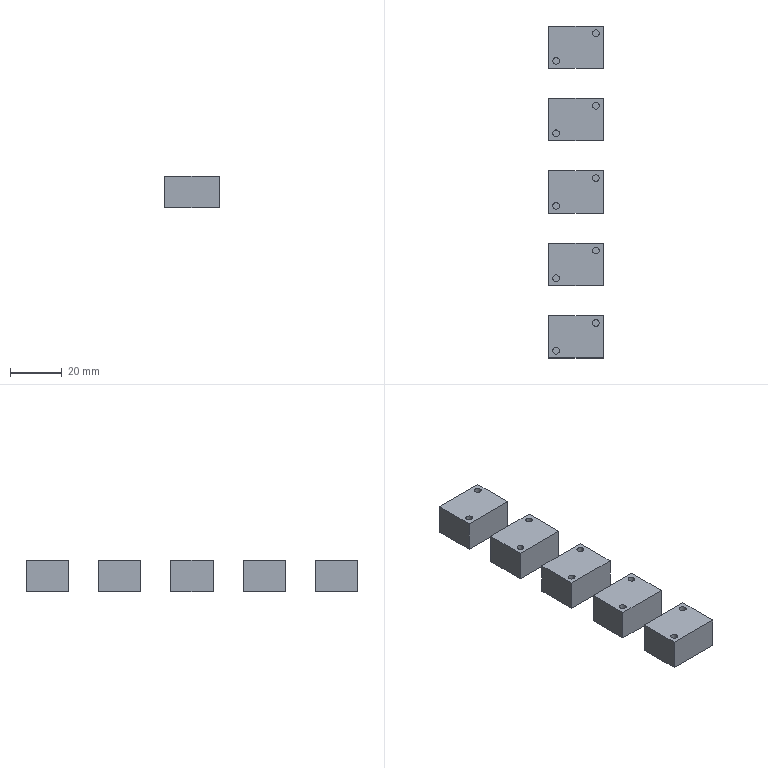NC program | NX | posted with a generic post | part box 21 x 128.262 x 12 mm
Lines 59 to 915 of 3295:
(ZLEVEL_PROFILE , TOOL : D10)
N104 T10 M6
N106 G54
N108 G17 G0 G90 X53.498 Y15.6 S9500 M3
N110 G43 Z30. H10
N112 Z1.5
N114 G94 G1 X64.131 Z0.943 F1000.
N116 X64.685 Z0.914
N118 X66.03 Y15.266 Z0.841
N120 X67.236 Y14.584 Z0.768
N122 X68.215 Y13.604 Z0.696
N124 X68.897 Y12.398 Z0.623
N126 X69.231 Y11.054 Z0.551
N128 Y-11.054 Z-0.608
N130 X68.897 Y-12.398 Z-0.681
N132 X68.215 Y-13.604 Z-0.753
N134 X67.236 Y-14.584 Z-0.826
N136 X66.03 Y-15.266 Z-0.898
N138 X64.685 Y-15.6 Z-0.971
N140 X64.131 Z-1.
N142 X47.869 F2500.
N144 G2 X42.769 Y-10.5 R5.1
N146 G1 Y10.5
N148 G2 X47.869 Y15.6 R5.1
N150 G1 X64.131
N152 G2 X69.231 Y10.5 R5.1
N154 G1 Y-10.5
N156 G2 X64.131 Y-15.6 R5.1
N158 G1 X47.873 Z-1.284
N160 X47.487 Y-15.586 Z-1.291
N162 X47.102 Y-15.542 Z-1.297
N164 X46.722 Y-15.469 Z-1.304
N166 X46.348 Y-15.368 Z-1.311
N168 X45.984 Y-15.239 Z-1.318
N170 X45.63 Y-15.082 Z-1.324
N172 X45.289 Y-14.899 Z-1.331
N174 X44.963 Y-14.691 Z-1.338
N176 X44.653 Y-14.458 Z-1.345
N178 X44.362 Y-14.203 Z-1.351
N180 X44.091 Y-13.927 Z-1.358
N182 X43.843 Y-13.63 Z-1.365
N184 X43.617 Y-13.316 Z-1.372
N186 X43.415 Y-12.986 Z-1.378
N188 X43.24 Y-12.641 Z-1.385
N190 X43.091 Y-12.284 Z-1.392
N192 X42.969 Y-11.916 Z-1.399
N194 X42.876 Y-11.54 Z-1.405
N196 X42.812 Y-11.159 Z-1.412
N198 X42.776 Y-10.774 Z-1.419
N200 X42.769 Y-10.387 Z-1.426
N202 Y-9.999 Z-1.432
N204 Y10.129 Z-1.784
N206 Y10.517 Z-1.791
N208 X42.785 Y10.903 Z-1.797
N210 X42.83 Y11.288 Z-1.804
N212 X42.904 Y11.667 Z-1.811
N214 X43.007 Y12.04 Z-1.818
N216 X43.138 Y12.405 Z-1.824
N218 X43.296 Y12.758 Z-1.831
N220 X43.48 Y13.098 Z-1.838
N222 X43.69 Y13.423 Z-1.845
N224 X43.924 Y13.732 Z-1.851
N226 X44.18 Y14.022 Z-1.858
N228 X44.458 Y14.291 Z-1.865
N230 X44.755 Y14.539 Z-1.872
N232 X45.07 Y14.764 Z-1.878
N234 X45.402 Y14.964 Z-1.885
N236 X45.747 Y15.138 Z-1.892
N238 X46.105 Y15.285 Z-1.899
N240 X46.473 Y15.405 Z-1.905
N242 X46.849 Y15.497 Z-1.912
N244 X47.231 Y15.56 Z-1.919
N246 X47.616 Y15.594 Z-1.926
N248 X48.003 Y15.6 Z-1.932
N250 X51.874 Z-2.
N252 X64.131
N254 G2 X69.231 Y10.5 R5.1
N256 G1 Y-10.5
N258 G2 X64.131 Y-15.6 R5.1
N260 G1 X47.873 Z-2.284
N262 X47.487 Y-15.586 Z-2.291
N264 X47.102 Y-15.542 Z-2.297
N266 X46.722 Y-15.469 Z-2.304
N268 X46.348 Y-15.368 Z-2.311
N270 X45.984 Y-15.239 Z-2.318
N272 X45.63 Y-15.082 Z-2.324
N274 X45.289 Y-14.899 Z-2.331
N276 X44.963 Y-14.691 Z-2.338
N278 X44.653 Y-14.458 Z-2.345
N280 X44.362 Y-14.203 Z-2.351
N282 X44.091 Y-13.927 Z-2.358
N284 X43.843 Y-13.63 Z-2.365
N286 X43.617 Y-13.316 Z-2.372
N288 X43.415 Y-12.986 Z-2.378
N290 X43.24 Y-12.641 Z-2.385
N292 X43.091 Y-12.284 Z-2.392
N294 X42.969 Y-11.916 Z-2.399
N296 X42.876 Y-11.54 Z-2.405
N298 X42.812 Y-11.159 Z-2.412
N300 X42.776 Y-10.774 Z-2.419
N302 X42.769 Y-10.387 Z-2.426
N304 Y-9.999 Z-2.432
N306 Y10.129 Z-2.784
N308 Y10.517 Z-2.791
N310 X42.785 Y10.903 Z-2.797
N312 X42.83 Y11.288 Z-2.804
N314 X42.904 Y11.667 Z-2.811
N316 X43.007 Y12.04 Z-2.818
N318 X43.138 Y12.405 Z-2.824
N320 X43.296 Y12.758 Z-2.831
N322 X43.48 Y13.098 Z-2.838
N324 X43.69 Y13.423 Z-2.845
N326 X43.924 Y13.732 Z-2.851
N328 X44.18 Y14.022 Z-2.858
N330 X44.458 Y14.291 Z-2.865
N332 X44.755 Y14.539 Z-2.872
N334 X45.07 Y14.764 Z-2.878
N336 X45.402 Y14.964 Z-2.885
N338 X45.747 Y15.138 Z-2.892
N340 X46.105 Y15.285 Z-2.899
N342 X46.473 Y15.405 Z-2.905
N344 X46.849 Y15.497 Z-2.912
N346 X47.231 Y15.56 Z-2.919
N348 X47.616 Y15.594 Z-2.926
N350 X48.003 Y15.6 Z-2.932
N352 X51.874 Z-3.
N354 X64.131
N356 G2 X69.231 Y10.5 R5.1
N358 G1 Y-10.5
N360 G2 X64.131 Y-15.6 R5.1
N362 G1 X47.873 Z-3.284
N364 X47.487 Y-15.586 Z-3.291
N366 X47.102 Y-15.542 Z-3.297
N368 X46.722 Y-15.469 Z-3.304
N370 X46.348 Y-15.368 Z-3.311
N372 X45.984 Y-15.239 Z-3.318
N374 X45.63 Y-15.082 Z-3.324
N376 X45.289 Y-14.899 Z-3.331
N378 X44.963 Y-14.691 Z-3.338
N380 X44.653 Y-14.458 Z-3.345
N382 X44.362 Y-14.203 Z-3.351
N384 X44.091 Y-13.927 Z-3.358
N386 X43.843 Y-13.63 Z-3.365
N388 X43.617 Y-13.316 Z-3.372
N390 X43.415 Y-12.986 Z-3.378
N392 X43.24 Y-12.641 Z-3.385
N394 X43.091 Y-12.284 Z-3.392
N396 X42.969 Y-11.916 Z-3.399
N398 X42.876 Y-11.54 Z-3.405
N400 X42.812 Y-11.159 Z-3.412
N402 X42.776 Y-10.774 Z-3.419
N404 X42.769 Y-10.387 Z-3.426
N406 Y-9.999 Z-3.432
N408 Y10.129 Z-3.784
N410 Y10.517 Z-3.791
N412 X42.785 Y10.903 Z-3.797
N414 X42.83 Y11.288 Z-3.804
N416 X42.904 Y11.667 Z-3.811
N418 X43.007 Y12.04 Z-3.818
N420 X43.138 Y12.405 Z-3.824
N422 X43.296 Y12.758 Z-3.831
N424 X43.48 Y13.098 Z-3.838
N426 X43.69 Y13.423 Z-3.845
N428 X43.924 Y13.732 Z-3.851
N430 X44.18 Y14.022 Z-3.858
N432 X44.458 Y14.291 Z-3.865
N434 X44.755 Y14.539 Z-3.872
N436 X45.07 Y14.764 Z-3.878
N438 X45.402 Y14.964 Z-3.885
N440 X45.747 Y15.138 Z-3.892
N442 X46.105 Y15.285 Z-3.899
N444 X46.473 Y15.405 Z-3.905
N446 X46.849 Y15.497 Z-3.912
N448 X47.231 Y15.56 Z-3.919
N450 X47.616 Y15.594 Z-3.926
N452 X48.003 Y15.6 Z-3.932
N454 X51.874 Z-4.
N456 X64.131
N458 G2 X69.231 Y10.5 R5.1
N460 G1 Y-10.5
N462 G2 X64.131 Y-15.6 R5.1
N464 G1 X47.873 Z-4.284
N466 X47.487 Y-15.586 Z-4.291
N468 X47.102 Y-15.542 Z-4.297
N470 X46.722 Y-15.469 Z-4.304
N472 X46.348 Y-15.368 Z-4.311
N474 X45.984 Y-15.239 Z-4.318
N476 X45.63 Y-15.082 Z-4.324
N478 X45.289 Y-14.899 Z-4.331
N480 X44.963 Y-14.691 Z-4.338
N482 X44.653 Y-14.458 Z-4.345
N484 X44.362 Y-14.203 Z-4.351
N486 X44.091 Y-13.927 Z-4.358
N488 X43.843 Y-13.63 Z-4.365
N490 X43.617 Y-13.316 Z-4.372
N492 X43.415 Y-12.986 Z-4.378
N494 X43.24 Y-12.641 Z-4.385
N496 X43.091 Y-12.284 Z-4.392
N498 X42.969 Y-11.916 Z-4.399
N500 X42.876 Y-11.54 Z-4.405
N502 X42.812 Y-11.159 Z-4.412
N504 X42.776 Y-10.774 Z-4.419
N506 X42.769 Y-10.387 Z-4.426
N508 Y-9.999 Z-4.432
N510 Y10.129 Z-4.784
N512 Y10.517 Z-4.791
N514 X42.785 Y10.903 Z-4.797
N516 X42.83 Y11.288 Z-4.804
N518 X42.904 Y11.667 Z-4.811
N520 X43.007 Y12.04 Z-4.818
N522 X43.138 Y12.405 Z-4.824
N524 X43.296 Y12.758 Z-4.831
N526 X43.48 Y13.098 Z-4.838
N528 X43.69 Y13.423 Z-4.845
N530 X43.924 Y13.732 Z-4.851
N532 X44.18 Y14.022 Z-4.858
N534 X44.458 Y14.291 Z-4.865
N536 X44.755 Y14.539 Z-4.872
N538 X45.07 Y14.764 Z-4.878
N540 X45.402 Y14.964 Z-4.885
N542 X45.747 Y15.138 Z-4.892
N544 X46.105 Y15.285 Z-4.899
N546 X46.473 Y15.405 Z-4.905
N548 X46.849 Y15.497 Z-4.912
N550 X47.231 Y15.56 Z-4.919
N552 X47.616 Y15.594 Z-4.926
N554 X48.003 Y15.6 Z-4.932
N556 X51.874 Z-5.
N558 X64.131
N560 G2 X69.231 Y10.5 R5.1
N562 G1 Y-10.5
N564 G2 X64.131 Y-15.6 R5.1
N566 G1 X47.873 Z-5.284
N568 X47.487 Y-15.586 Z-5.291
N570 X47.102 Y-15.542 Z-5.297
N572 X46.722 Y-15.469 Z-5.304
N574 X46.348 Y-15.368 Z-5.311
N576 X45.984 Y-15.239 Z-5.318
N578 X45.63 Y-15.082 Z-5.324
N580 X45.289 Y-14.899 Z-5.331
N582 X44.963 Y-14.691 Z-5.338
N584 X44.653 Y-14.458 Z-5.345
N586 X44.362 Y-14.203 Z-5.351
N588 X44.091 Y-13.927 Z-5.358
N590 X43.843 Y-13.63 Z-5.365
N592 X43.617 Y-13.316 Z-5.372
N594 X43.415 Y-12.986 Z-5.378
N596 X43.24 Y-12.641 Z-5.385
N598 X43.091 Y-12.284 Z-5.392
N600 X42.969 Y-11.916 Z-5.399
N602 X42.876 Y-11.54 Z-5.405
N604 X42.812 Y-11.159 Z-5.412
N606 X42.776 Y-10.774 Z-5.419
N608 X42.769 Y-10.387 Z-5.426
N610 Y-9.999 Z-5.432
N612 Y10.129 Z-5.784
N614 Y10.517 Z-5.791
N616 X42.785 Y10.903 Z-5.797
N618 X42.83 Y11.288 Z-5.804
N620 X42.904 Y11.667 Z-5.811
N622 X43.007 Y12.04 Z-5.818
N624 X43.138 Y12.405 Z-5.824
N626 X43.296 Y12.758 Z-5.831
N628 X43.48 Y13.098 Z-5.838
N630 X43.69 Y13.423 Z-5.845
N632 X43.924 Y13.732 Z-5.851
N634 X44.18 Y14.022 Z-5.858
N636 X44.458 Y14.291 Z-5.865
N638 X44.755 Y14.539 Z-5.872
N640 X45.07 Y14.764 Z-5.878
N642 X45.402 Y14.964 Z-5.885
N644 X45.747 Y15.138 Z-5.892
N646 X46.105 Y15.285 Z-5.899
N648 X46.473 Y15.405 Z-5.905
N650 X46.849 Y15.497 Z-5.912
N652 X47.231 Y15.56 Z-5.919
N654 X47.616 Y15.594 Z-5.926
N656 X48.003 Y15.6 Z-5.932
N658 X51.874 Z-6.
N660 X64.131
N662 G2 X69.231 Y10.5 R5.1
N664 G1 Y-10.5
N666 G2 X64.131 Y-15.6 R5.1
N668 G1 X47.873 Z-6.284
N670 X47.487 Y-15.586 Z-6.291
N672 X47.102 Y-15.542 Z-6.297
N674 X46.722 Y-15.469 Z-6.304
N676 X46.348 Y-15.368 Z-6.311
N678 X45.984 Y-15.239 Z-6.318
N680 X45.63 Y-15.082 Z-6.324
N682 X45.289 Y-14.899 Z-6.331
N684 X44.963 Y-14.691 Z-6.338
N686 X44.653 Y-14.458 Z-6.345
N688 X44.362 Y-14.203 Z-6.351
N690 X44.091 Y-13.927 Z-6.358
N692 X43.843 Y-13.63 Z-6.365
N694 X43.617 Y-13.316 Z-6.372
N696 X43.415 Y-12.986 Z-6.378
N698 X43.24 Y-12.641 Z-6.385
N700 X43.091 Y-12.284 Z-6.392
N702 X42.969 Y-11.916 Z-6.399
N704 X42.876 Y-11.54 Z-6.405
N706 X42.812 Y-11.159 Z-6.412
N708 X42.776 Y-10.774 Z-6.419
N710 X42.769 Y-10.387 Z-6.426
N712 Y-9.999 Z-6.432
N714 Y10.129 Z-6.784
N716 Y10.517 Z-6.791
N718 X42.785 Y10.903 Z-6.797
N720 X42.83 Y11.288 Z-6.804
N722 X42.904 Y11.667 Z-6.811
N724 X43.007 Y12.04 Z-6.818
N726 X43.138 Y12.405 Z-6.824
N728 X43.296 Y12.758 Z-6.831
N730 X43.48 Y13.098 Z-6.838
N732 X43.69 Y13.423 Z-6.845
N734 X43.924 Y13.732 Z-6.851
N736 X44.18 Y14.022 Z-6.858
N738 X44.458 Y14.291 Z-6.865
N740 X44.755 Y14.539 Z-6.872
N742 X45.07 Y14.764 Z-6.878
N744 X45.402 Y14.964 Z-6.885
N746 X45.747 Y15.138 Z-6.892
N748 X46.105 Y15.285 Z-6.899
N750 X46.473 Y15.405 Z-6.905
N752 X46.849 Y15.497 Z-6.912
N754 X47.231 Y15.56 Z-6.919
N756 X47.616 Y15.594 Z-6.926
N758 X48.003 Y15.6 Z-6.932
N760 X51.874 Z-7.
N762 X64.131
N764 G2 X69.231 Y10.5 R5.1
N766 G1 Y-10.5
N768 G2 X64.131 Y-15.6 R5.1
N770 G1 X47.873 Z-7.284
N772 X47.487 Y-15.586 Z-7.291
N774 X47.102 Y-15.542 Z-7.297
N776 X46.722 Y-15.469 Z-7.304
N778 X46.348 Y-15.368 Z-7.311
N780 X45.984 Y-15.239 Z-7.318
N782 X45.63 Y-15.082 Z-7.324
N784 X45.289 Y-14.899 Z-7.331
N786 X44.963 Y-14.691 Z-7.338
N788 X44.653 Y-14.458 Z-7.345
N790 X44.362 Y-14.203 Z-7.351
N792 X44.091 Y-13.927 Z-7.358
N794 X43.843 Y-13.63 Z-7.365
N796 X43.617 Y-13.316 Z-7.372
N798 X43.415 Y-12.986 Z-7.378
N800 X43.24 Y-12.641 Z-7.385
N802 X43.091 Y-12.284 Z-7.392
N804 X42.969 Y-11.916 Z-7.399
N806 X42.876 Y-11.54 Z-7.405
N808 X42.812 Y-11.159 Z-7.412
N810 X42.776 Y-10.774 Z-7.419
N812 X42.769 Y-10.387 Z-7.426
N814 Y-9.999 Z-7.432
N816 Y10.129 Z-7.784
N818 Y10.517 Z-7.791
N820 X42.785 Y10.903 Z-7.797
N822 X42.83 Y11.288 Z-7.804
N824 X42.904 Y11.667 Z-7.811
N826 X43.007 Y12.04 Z-7.818
N828 X43.138 Y12.405 Z-7.824
N830 X43.296 Y12.758 Z-7.831
N832 X43.48 Y13.098 Z-7.838
N834 X43.69 Y13.423 Z-7.845
N836 X43.924 Y13.732 Z-7.851
N838 X44.18 Y14.022 Z-7.858
N840 X44.458 Y14.291 Z-7.865
N842 X44.755 Y14.539 Z-7.872
N844 X45.07 Y14.764 Z-7.878
N846 X45.402 Y14.964 Z-7.885
N848 X45.747 Y15.138 Z-7.892
N850 X46.105 Y15.285 Z-7.899
N852 X46.473 Y15.405 Z-7.905
N854 X46.849 Y15.497 Z-7.912
N856 X47.231 Y15.56 Z-7.919
N858 X47.616 Y15.594 Z-7.926
N860 X48.003 Y15.6 Z-7.932
N862 X51.874 Z-8.
N864 X64.131
N866 G2 X69.231 Y10.5 R5.1
N868 G1 Y-10.5
N870 G2 X64.131 Y-15.6 R5.1
N872 G1 X47.873 Z-8.284
N874 X47.487 Y-15.586 Z-8.291
N876 X47.102 Y-15.542 Z-8.297
N878 X46.722 Y-15.469 Z-8.304
N880 X46.348 Y-15.368 Z-8.311
N882 X45.984 Y-15.239 Z-8.318
N884 X45.63 Y-15.082 Z-8.324
N886 X45.289 Y-14.899 Z-8.331
N888 X44.963 Y-14.691 Z-8.338
N890 X44.653 Y-14.458 Z-8.345
N892 X44.362 Y-14.203 Z-8.351
N894 X44.091 Y-13.927 Z-8.358
N896 X43.843 Y-13.63 Z-8.365
N898 X43.617 Y-13.316 Z-8.372
N900 X43.415 Y-12.986 Z-8.378
N902 X43.24 Y-12.641 Z-8.385
N904 X43.091 Y-12.284 Z-8.392
N906 X42.969 Y-11.916 Z-8.399
N908 X42.876 Y-11.54 Z-8.405
N910 X42.812 Y-11.159 Z-8.412
N912 X42.776 Y-10.774 Z-8.419
N914 X42.769 Y-10.387 Z-8.426
N916 Y-9.999 Z-8.432
N918 Y10.129 Z-8.784
N920 Y10.517 Z-8.791
N922 X42.785 Y10.903 Z-8.797
N924 X42.83 Y11.288 Z-8.804
N926 X42.904 Y11.667 Z-8.811
N928 X43.007 Y12.04 Z-8.818
N930 X43.138 Y12.405 Z-8.824
N932 X43.296 Y12.758 Z-8.831
N934 X43.48 Y13.098 Z-8.838
N936 X43.69 Y13.423 Z-8.845
N938 X43.924 Y13.732 Z-8.851
N940 X44.18 Y14.022 Z-8.858
N942 X44.458 Y14.291 Z-8.865
N944 X44.755 Y14.539 Z-8.872
N946 X45.07 Y14.764 Z-8.878
N948 X45.402 Y14.964 Z-8.885
N950 X45.747 Y15.138 Z-8.892
N952 X46.105 Y15.285 Z-8.899
N954 X46.473 Y15.405 Z-8.905
N956 X46.849 Y15.497 Z-8.912
N958 X47.231 Y15.56 Z-8.919
N960 X47.616 Y15.594 Z-8.926
N962 X48.003 Y15.6 Z-8.932
N964 X51.874 Z-9.
N966 X64.131
N968 G2 X69.231 Y10.5 R5.1
N970 G1 Y-10.5
N972 G2 X64.131 Y-15.6 R5.1
N974 G1 X47.873 Z-9.284
N976 X47.487 Y-15.586 Z-9.291
N978 X47.102 Y-15.542 Z-9.297
N980 X46.722 Y-15.469 Z-9.304
N982 X46.348 Y-15.368 Z-9.311
N984 X45.984 Y-15.239 Z-9.318
N986 X45.63 Y-15.082 Z-9.324
N988 X45.289 Y-14.899 Z-9.331
N990 X44.963 Y-14.691 Z-9.338
N992 X44.653 Y-14.458 Z-9.345
N994 X44.362 Y-14.203 Z-9.351
N996 X44.091 Y-13.927 Z-9.358
N998 X43.843 Y-13.63 Z-9.365
N1000 X43.617 Y-13.316 Z-9.372
N1002 X43.415 Y-12.986 Z-9.378
N1004 X43.24 Y-12.641 Z-9.385
N1006 X43.091 Y-12.284 Z-9.392
N1008 X42.969 Y-11.916 Z-9.399
N1010 X42.876 Y-11.54 Z-9.405
N1012 X42.812 Y-11.159 Z-9.412
N1014 X42.776 Y-10.774 Z-9.419
N1016 X42.769 Y-10.387 Z-9.426
N1018 Y-9.999 Z-9.432
N1020 Y10.129 Z-9.784
N1022 Y10.517 Z-9.791
N1024 X42.785 Y10.903 Z-9.797
N1026 X42.83 Y11.288 Z-9.804
N1028 X42.904 Y11.667 Z-9.811
N1030 X43.007 Y12.04 Z-9.818
N1032 X43.138 Y12.405 Z-9.824
N1034 X43.296 Y12.758 Z-9.831
N1036 X43.48 Y13.098 Z-9.838
N1038 X43.69 Y13.423 Z-9.845
N1040 X43.924 Y13.732 Z-9.851
N1042 X44.18 Y14.022 Z-9.858
N1044 X44.458 Y14.291 Z-9.865
N1046 X44.755 Y14.539 Z-9.872
N1048 X45.07 Y14.764 Z-9.878
N1050 X45.402 Y14.964 Z-9.885
N1052 X45.747 Y15.138 Z-9.892
N1054 X46.105 Y15.285 Z-9.899
N1056 X46.473 Y15.405 Z-9.905
N1058 X46.849 Y15.497 Z-9.912
N1060 X47.231 Y15.56 Z-9.919
N1062 X47.616 Y15.594 Z-9.926
N1064 X48.003 Y15.6 Z-9.932
N1066 X51.874 Z-10.
N1068 X64.131
N1070 G2 X69.231 Y10.5 R5.1
N1072 G1 Y-10.5
N1074 G2 X64.131 Y-15.6 R5.1
N1076 G1 X47.873 Z-10.284
N1078 X47.487 Y-15.586 Z-10.291
N1080 X47.102 Y-15.542 Z-10.297
N1082 X46.722 Y-15.469 Z-10.304
N1084 X46.348 Y-15.368 Z-10.311
N1086 X45.984 Y-15.239 Z-10.318
N1088 X45.63 Y-15.082 Z-10.324
N1090 X45.289 Y-14.899 Z-10.331
N1092 X44.963 Y-14.691 Z-10.338
N1094 X44.653 Y-14.458 Z-10.345
N1096 X44.362 Y-14.203 Z-10.351
N1098 X44.091 Y-13.927 Z-10.358
N1100 X43.843 Y-13.63 Z-10.365
N1102 X43.617 Y-13.316 Z-10.372
N1104 X43.415 Y-12.986 Z-10.378
N1106 X43.24 Y-12.641 Z-10.385
N1108 X43.091 Y-12.284 Z-10.392
N1110 X42.969 Y-11.916 Z-10.399
N1112 X42.876 Y-11.54 Z-10.405
N1114 X42.812 Y-11.159 Z-10.412
N1116 X42.776 Y-10.774 Z-10.419
N1118 X42.769 Y-10.387 Z-10.426
N1120 Y-9.999 Z-10.432
N1122 Y10.129 Z-10.784
N1124 Y10.517 Z-10.791
N1126 X42.785 Y10.903 Z-10.797
N1128 X42.83 Y11.288 Z-10.804
N1130 X42.904 Y11.667 Z-10.811
N1132 X43.007 Y12.04 Z-10.818
N1134 X43.138 Y12.405 Z-10.824
N1136 X43.296 Y12.758 Z-10.831
N1138 X43.48 Y13.098 Z-10.838
N1140 X43.69 Y13.423 Z-10.845
N1142 X43.924 Y13.732 Z-10.851
N1144 X44.18 Y14.022 Z-10.858
N1146 X44.458 Y14.291 Z-10.865
N1148 X44.755 Y14.539 Z-10.872
N1150 X45.07 Y14.764 Z-10.878
N1152 X45.402 Y14.964 Z-10.885
N1154 X45.747 Y15.138 Z-10.892
N1156 X46.105 Y15.285 Z-10.899
N1158 X46.473 Y15.405 Z-10.905
N1160 X46.849 Y15.497 Z-10.912
N1162 X47.231 Y15.56 Z-10.919
N1164 X47.616 Y15.594 Z-10.926
N1166 X48.003 Y15.6 Z-10.932
N1168 X51.874 Z-11.
N1170 X64.131
N1172 G2 X69.231 Y10.5 R5.1
N1174 G1 Y-10.5
N1176 G2 X64.131 Y-15.6 R5.1
N1178 G1 X47.873 Z-11.284
N1180 X47.487 Y-15.586 Z-11.291
N1182 X47.102 Y-15.542 Z-11.297
N1184 X46.722 Y-15.469 Z-11.304
N1186 X46.348 Y-15.368 Z-11.311
N1188 X45.984 Y-15.239 Z-11.318
N1190 X45.63 Y-15.082 Z-11.324
N1192 X45.289 Y-14.899 Z-11.331
N1194 X44.963 Y-14.691 Z-11.338
N1196 X44.653 Y-14.458 Z-11.345
N1198 X44.362 Y-14.203 Z-11.351
N1200 X44.091 Y-13.927 Z-11.358
N1202 X43.843 Y-13.63 Z-11.365
N1204 X43.617 Y-13.316 Z-11.372
N1206 X43.415 Y-12.986 Z-11.378
N1208 X43.24 Y-12.641 Z-11.385
N1210 X43.091 Y-12.284 Z-11.392
N1212 X42.969 Y-11.916 Z-11.399
N1214 X42.876 Y-11.54 Z-11.405
N1216 X42.812 Y-11.159 Z-11.412
N1218 X42.776 Y-10.774 Z-11.419
N1220 X42.769 Y-10.387 Z-11.426
N1222 Y-9.999 Z-11.432
N1224 Y10.129 Z-11.784
N1226 Y10.517 Z-11.791
N1228 X42.785 Y10.903 Z-11.797
N1230 X42.83 Y11.288 Z-11.804
N1232 X42.904 Y11.667 Z-11.811
N1234 X43.007 Y12.04 Z-11.818
N1236 X43.138 Y12.405 Z-11.824
N1238 X43.296 Y12.758 Z-11.831
N1240 X43.48 Y13.098 Z-11.838
N1242 X43.69 Y13.423 Z-11.845
N1244 X43.924 Y13.732 Z-11.851
N1246 X44.18 Y14.022 Z-11.858
N1248 X44.458 Y14.291 Z-11.865
N1250 X44.755 Y14.539 Z-11.872
N1252 X45.07 Y14.764 Z-11.878
N1254 X45.402 Y14.964 Z-11.885
N1256 X45.747 Y15.138 Z-11.892
N1258 X46.105 Y15.285 Z-11.899
N1260 X46.473 Y15.405 Z-11.905
N1262 X46.849 Y15.497 Z-11.912
N1264 X47.231 Y15.56 Z-11.919
N1266 X47.616 Y15.594 Z-11.926
N1268 X48.003 Y15.6 Z-11.932
N1270 X51.874 Z-12.
N1272 X64.131
N1274 G2 X69.231 Y10.5 R5.1
N1276 G1 Y-10.5
N1278 G2 X64.131 Y-15.6 R5.1
N1280 G1 X47.869
N1282 G2 X42.769 Y-10.5 R5.1
N1284 G1 Y10.5
N1286 G2 X47.869 Y15.6 R5.1
N1288 G1 X51.874
N1290 Z-10.5
N1292 G0 Z30.
N1294 X25.498
N1296 Z1.5
N1298 G1 X36.131 Z0.943 F1000.
N1300 X36.685 Z0.914
N1302 X38.03 Y15.266 Z0.841
N1304 X39.236 Y14.584 Z0.768
N1306 X40.215 Y13.604 Z0.696
N1308 X40.897 Y12.398 Z0.623
N1310 X41.231 Y11.054 Z0.551
N1312 Y-11.054 Z-0.608
N1314 X40.897 Y-12.398 Z-0.681
N1316 X40.215 Y-13.604 Z-0.753
N1318 X39.236 Y-14.584 Z-0.826
N1320 X38.03 Y-15.266 Z-0.898
N1322 X36.685 Y-15.6 Z-0.971
N1324 X36.131 Z-1.
N1326 X19.869 F2500.
N1328 G2 X14.769 Y-10.5 R5.1
N1330 G1 Y10.5
N1332 G2 X19.869 Y15.6 R5.1
N1334 G1 X36.131
N1336 G2 X41.231 Y10.5 R5.1
N1338 G1 Y-10.5
N1340 G2 X36.131 Y-15.6 R5.1
N1342 G1 X19.873 Z-1.284
N1344 X19.487 Y-15.586 Z-1.291
N1346 X19.102 Y-15.542 Z-1.297
N1348 X18.722 Y-15.469 Z-1.304
N1350 X18.348 Y-15.368 Z-1.311
N1352 X17.984 Y-15.239 Z-1.318
N1354 X17.63 Y-15.082 Z-1.324
N1356 X17.289 Y-14.899 Z-1.331
N1358 X16.963 Y-14.691 Z-1.338
N1360 X16.653 Y-14.458 Z-1.345
N1362 X16.362 Y-14.203 Z-1.351
N1364 X16.091 Y-13.927 Z-1.358
N1366 X15.843 Y-13.63 Z-1.365
N1368 X15.617 Y-13.316 Z-1.372
N1370 X15.415 Y-12.986 Z-1.378
N1372 X15.24 Y-12.641 Z-1.385
N1374 X15.091 Y-12.284 Z-1.392
N1376 X14.969 Y-11.916 Z-1.399
N1378 X14.876 Y-11.541 Z-1.405
N1380 X14.812 Y-11.159 Z-1.412
N1382 X14.776 Y-10.774 Z-1.419
N1384 X14.769 Y-10.387 Z-1.426
N1386 Y-9.999 Z-1.432
N1388 Y10.129 Z-1.784
N1390 Y10.517 Z-1.791
N1392 X14.785 Y10.903 Z-1.797
N1394 X14.83 Y11.288 Z-1.804
N1396 X14.904 Y11.667 Z-1.811
N1398 X15.007 Y12.04 Z-1.818
N1400 X15.138 Y12.405 Z-1.824
N1402 X15.296 Y12.758 Z-1.831
N1404 X15.48 Y13.098 Z-1.838
N1406 X15.69 Y13.423 Z-1.845
N1408 X15.924 Y13.732 Z-1.851
N1410 X16.18 Y14.022 Z-1.858
N1412 X16.458 Y14.291 Z-1.865
N1414 X16.755 Y14.539 Z-1.872
N1416 X17.07 Y14.764 Z-1.878
N1418 X17.402 Y14.964 Z-1.885
N1420 X17.747 Y15.138 Z-1.892
N1422 X18.105 Y15.285 Z-1.899
N1424 X18.473 Y15.405 Z-1.905
N1426 X18.849 Y15.497 Z-1.912
N1428 X19.231 Y15.56 Z-1.919
N1430 X19.616 Y15.594 Z-1.926
N1432 X20.003 Y15.6 Z-1.932
N1434 X23.874 Z-2.
N1436 X36.131
N1438 G2 X41.231 Y10.5 R5.1
N1440 G1 Y-10.5
N1442 G2 X36.131 Y-15.6 R5.1
N1444 G1 X19.873 Z-2.284
N1446 X19.487 Y-15.586 Z-2.291
N1448 X19.102 Y-15.542 Z-2.297
N1450 X18.722 Y-15.469 Z-2.304
N1452 X18.348 Y-15.368 Z-2.311
N1454 X17.984 Y-15.239 Z-2.318
N1456 X17.63 Y-15.082 Z-2.324
N1458 X17.289 Y-14.899 Z-2.331
N1460 X16.963 Y-14.691 Z-2.338
N1462 X16.653 Y-14.458 Z-2.345
N1464 X16.362 Y-14.203 Z-2.351
N1466 X16.091 Y-13.927 Z-2.358
N1468 X15.843 Y-13.63 Z-2.365
N1470 X15.617 Y-13.316 Z-2.372
N1472 X15.415 Y-12.986 Z-2.378
N1474 X15.24 Y-12.641 Z-2.385
N1476 X15.091 Y-12.284 Z-2.392
N1478 X14.969 Y-11.916 Z-2.399
N1480 X14.876 Y-11.541 Z-2.405
N1482 X14.812 Y-11.159 Z-2.412
N1484 X14.776 Y-10.774 Z-2.419
N1486 X14.769 Y-10.387 Z-2.426
N1488 Y-9.999 Z-2.432
N1490 Y10.129 Z-2.784
N1492 Y10.517 Z-2.791
N1494 X14.785 Y10.903 Z-2.797
N1496 X14.83 Y11.288 Z-2.804
N1498 X14.904 Y11.667 Z-2.811
N1500 X15.007 Y12.04 Z-2.818
N1502 X15.138 Y12.405 Z-2.824
N1504 X15.296 Y12.758 Z-2.831
N1506 X15.48 Y13.098 Z-2.838
N1508 X15.69 Y13.423 Z-2.845
N1510 X15.924 Y13.732 Z-2.851
N1512 X16.18 Y14.022 Z-2.858
N1514 X16.458 Y14.291 Z-2.865
N1516 X16.755 Y14.539 Z-2.872
N1518 X17.07 Y14.764 Z-2.878
N1520 X17.402 Y14.964 Z-2.885
N1522 X17.747 Y15.138 Z-2.892
N1524 X18.105 Y15.285 Z-2.899
N1526 X18.473 Y15.405 Z-2.905
N1528 X18.849 Y15.497 Z-2.912
N1530 X19.231 Y15.56 Z-2.919
N1532 X19.616 Y15.594 Z-2.926
N1534 X20.003 Y15.6 Z-2.932
N1536 X23.874 Z-3.
N1538 X36.131
N1540 G2 X41.231 Y10.5 R5.1
N1542 G1 Y-10.5
N1544 G2 X36.131 Y-15.6 R5.1
N1546 G1 X19.873 Z-3.284
N1548 X19.487 Y-15.586 Z-3.291
N1550 X19.102 Y-15.542 Z-3.297
N1552 X18.722 Y-15.469 Z-3.304
N1554 X18.348 Y-15.368 Z-3.311
N1556 X17.984 Y-15.239 Z-3.318
N1558 X17.63 Y-15.082 Z-3.324
N1560 X17.289 Y-14.899 Z-3.331
N1562 X16.963 Y-14.691 Z-3.338
N1564 X16.653 Y-14.458 Z-3.345
N1566 X16.362 Y-14.203 Z-3.351
N1568 X16.091 Y-13.927 Z-3.358
N1570 X15.843 Y-13.63 Z-3.365
N1572 X15.617 Y-13.316 Z-3.372
N1574 X15.415 Y-12.986 Z-3.378
N1576 X15.24 Y-12.641 Z-3.385
N1578 X15.091 Y-12.284 Z-3.392
N1580 X14.969 Y-11.916 Z-3.399
N1582 X14.876 Y-11.541 Z-3.405
N1584 X14.812 Y-11.159 Z-3.412
N1586 X14.776 Y-10.774 Z-3.419
N1588 X14.769 Y-10.387 Z-3.426
N1590 Y-9.999 Z-3.432
N1592 Y10.129 Z-3.784
N1594 Y10.517 Z-3.791
N1596 X14.785 Y10.903 Z-3.797
N1598 X14.83 Y11.288 Z-3.804
N1600 X14.904 Y11.667 Z-3.811
N1602 X15.007 Y12.04 Z-3.818
N1604 X15.138 Y12.405 Z-3.824
N1606 X15.296 Y12.758 Z-3.831
N1608 X15.48 Y13.098 Z-3.838
N1610 X15.69 Y13.423 Z-3.845
N1612 X15.924 Y13.732 Z-3.851
N1614 X16.18 Y14.022 Z-3.858
N1616 X16.458 Y14.291 Z-3.865
N1618 X16.755 Y14.539 Z-3.872
N1620 X17.07 Y14.764 Z-3.878
N1622 X17.402 Y14.964 Z-3.885
N1624 X17.747 Y15.138 Z-3.892
N1626 X18.105 Y15.285 Z-3.899
N1628 X18.473 Y15.405 Z-3.905
N1630 X18.849 Y15.497 Z-3.912
N1632 X19.231 Y15.56 Z-3.919
N1634 X19.616 Y15.594 Z-3.926
N1636 X20.003 Y15.6 Z-3.932
N1638 X23.874 Z-4.
N1640 X36.131
N1642 G2 X41.231 Y10.5 R5.1
N1644 G1 Y-10.5
N1646 G2 X36.131 Y-15.6 R5.1
N1648 G1 X19.873 Z-4.284
N1650 X19.487 Y-15.586 Z-4.291
N1652 X19.102 Y-15.542 Z-4.297
N1654 X18.722 Y-15.469 Z-4.304
N1656 X18.348 Y-15.368 Z-4.311
N1658 X17.984 Y-15.239 Z-4.318
N1660 X17.63 Y-15.082 Z-4.324
N1662 X17.289 Y-14.899 Z-4.331
N1664 X16.963 Y-14.691 Z-4.338
N1666 X16.653 Y-14.458 Z-4.345
N1668 X16.362 Y-14.203 Z-4.351
N1670 X16.091 Y-13.927 Z-4.358
N1672 X15.843 Y-13.63 Z-4.365
N1674 X15.617 Y-13.316 Z-4.372
N1676 X15.415 Y-12.986 Z-4.378
N1678 X15.24 Y-12.641 Z-4.385
N1680 X15.091 Y-12.284 Z-4.392
N1682 X14.969 Y-11.916 Z-4.399
N1684 X14.876 Y-11.541 Z-4.405
N1686 X14.812 Y-11.159 Z-4.412
N1688 X14.776 Y-10.774 Z-4.419
N1690 X14.769 Y-10.387 Z-4.426
N1692 Y-9.999 Z-4.432
N1694 Y10.129 Z-4.784
N1696 Y10.517 Z-4.791
N1698 X14.785 Y10.903 Z-4.797
N1700 X14.83 Y11.288 Z-4.804
N1702 X14.904 Y11.667 Z-4.811
N1704 X15.007 Y12.04 Z-4.818
N1706 X15.138 Y12.405 Z-4.824
N1708 X15.296 Y12.758 Z-4.831
N1710 X15.48 Y13.098 Z-4.838
N1712 X15.69 Y13.423 Z-4.845
N1714 X15.924 Y13.732 Z-4.851
N1716 X16.18 Y14.022 Z-4.858
N1718 X16.458 Y14.291 Z-4.865
N1720 X16.755 Y14.539 Z-4.872
N1722 X17.07 Y14.764 Z-4.878
N1724 X17.402 Y14.964 Z-4.885
N1726 X17.747 Y15.138 Z-4.892
N1728 X18.105 Y15.285 Z-4.899
N1730 X18.473 Y15.405 Z-4.905
N1732 X18.849 Y15.497 Z-4.912
N1734 X19.231 Y15.56 Z-4.919
N1736 X19.616 Y15.594 Z-4.926
N1738 X20.003 Y15.6 Z-4.932
N1740 X23.874 Z-5.
N1742 X36.131
N1744 G2 X41.231 Y10.5 R5.1
N1746 G1 Y-10.5
N1748 G2 X36.131 Y-15.6 R5.1
N1750 G1 X19.873 Z-5.284
N1752 X19.487 Y-15.586 Z-5.291
N1754 X19.102 Y-15.542 Z-5.297
N1756 X18.722 Y-15.469 Z-5.304
N1758 X18.348 Y-15.368 Z-5.311
N1760 X17.984 Y-15.239 Z-5.318
N1762 X17.63 Y-15.082 Z-5.324
N1764 X17.289 Y-14.899 Z-5.331
N1766 X16.963 Y-14.691 Z-5.338
N1768 X16.653 Y-14.458 Z-5.345
N1770 X16.362 Y-14.203 Z-5.351
N1772 X16.091 Y-13.927 Z-5.358
N1774 X15.843 Y-13.63 Z-5.365
N1776 X15.617 Y-13.316 Z-5.372
N1778 X15.415 Y-12.986 Z-5.378
N1780 X15.24 Y-12.641 Z-5.385
N1782 X15.091 Y-12.284 Z-5.392
N1784 X14.969 Y-11.916 Z-5.399
N1786 X14.876 Y-11.541 Z-5.405
N1788 X14.812 Y-11.159 Z-5.412
N1790 X14.776 Y-10.774 Z-5.419
N1792 X14.769 Y-10.387 Z-5.426
N1794 Y-9.999 Z-5.432
N1796 Y10.129 Z-5.784
N1798 Y10.517 Z-5.791
N1800 X14.785 Y10.903 Z-5.797
N1802 X14.83 Y11.288 Z-5.804
N1804 X14.904 Y11.667 Z-5.811
N1806 X15.007 Y12.04 Z-5.818
N1808 X15.138 Y12.405 Z-5.824
N1810 X15.296 Y12.758 Z-5.831